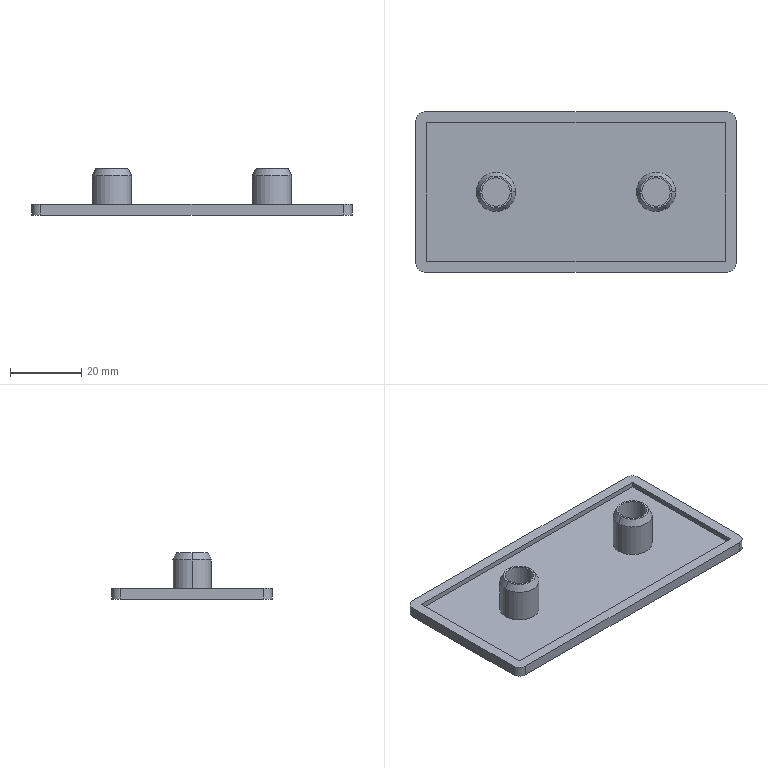Part | STEP file | HFC8_4590_Bc | 1 solid | 31 faces | box 90 x 45 x 13 mm | volume 8335 mm3 | plane 15 | cylinder 12 | cone 4 | commonest cylinder face diameters 5 x4 8 x4 11 x4
STEP:
#1=CARTESIAN_POINT('',(28.,0.,-1.5));
#2=VERTEX_POINT('',#1);
#3=CARTESIAN_POINT('',(17.,0.,-1.5));
#4=VERTEX_POINT('',#3);
#5=CARTESIAN_POINT('',(22.5,0.,-1.5));
#6=DIRECTION('',(0.,0.,1.));
#7=DIRECTION('',(1.,0.,0.));
#8=AXIS2_PLACEMENT_3D('',#5,#6,#7);
#9=CIRCLE('',#8,5.5);
#10=EDGE_CURVE('',#2,#4,#9,.T.);
#11=ORIENTED_EDGE('',*,*,#10,.T.);
#12=CARTESIAN_POINT('',(17.,0.,8.));
#13=VERTEX_POINT('',#12);
#14=CARTESIAN_POINT('',(17.,0.,-1.5));
#15=DIRECTION('',(0.,0.,1.));
#16=VECTOR('',#15,1000.);
#17=LINE('',#14,#16);
#18=EDGE_CURVE('',#4,#13,#17,.T.);
#19=ORIENTED_EDGE('',*,*,#18,.T.);
#20=CARTESIAN_POINT('',(28.,0.,8.));
#21=VERTEX_POINT('',#20);
#22=CARTESIAN_POINT('',(22.5,0.,8.));
#23=DIRECTION('',(0.,0.,1.));
#24=DIRECTION('',(1.,0.,0.));
#25=AXIS2_PLACEMENT_3D('',#22,#23,#24);
#26=CIRCLE('',#25,5.5);
#27=EDGE_CURVE('',#21,#13,#26,.T.);
#28=ORIENTED_EDGE('',*,*,#27,.F.);
#29=CARTESIAN_POINT('',(28.,0.,-1.5));
#30=DIRECTION('',(0.,0.,1.));
#31=VECTOR('',#30,1000.);
#32=LINE('',#29,#31);
#33=EDGE_CURVE('',#2,#21,#32,.T.);
#34=ORIENTED_EDGE('',*,*,#33,.F.);
#35=EDGE_LOOP('',(#11,#19,#28,#34));
#36=FACE_OUTER_BOUND('',#35,.T.);
#37=CARTESIAN_POINT('',(22.5,0.,-1.5));
#38=DIRECTION('',(0.,0.,1.));
#39=DIRECTION('',(1.,0.,0.));
#40=AXIS2_PLACEMENT_3D('',#37,#38,#39);
#41=CYLINDRICAL_SURFACE('',#40,5.5);
#42=ADVANCED_FACE('',(#36),#41,.T.);
#43=CARTESIAN_POINT('',(27.,0.,10.));
#44=VERTEX_POINT('',#43);
#45=CARTESIAN_POINT('',(18.,0.,10.));
#46=VERTEX_POINT('',#45);
#47=CARTESIAN_POINT('',(22.5,0.,10.));
#48=DIRECTION('',(0.,0.,1.));
#49=DIRECTION('',(1.,0.,0.));
#50=AXIS2_PLACEMENT_3D('',#47,#48,#49);
#51=CIRCLE('',#50,4.5);
#52=EDGE_CURVE('',#44,#46,#51,.T.);
#53=ORIENTED_EDGE('',*,*,#52,.F.);
#54=CARTESIAN_POINT('',(28.,0.,8.));
#55=DIRECTION('',(0.4472,0.,-0.8944));
#56=VECTOR('',#55,1000.);
#57=LINE('',#54,#56);
#58=EDGE_CURVE('',#44,#21,#57,.T.);
#59=ORIENTED_EDGE('',*,*,#58,.T.);
#60=ORIENTED_EDGE('',*,*,#27,.T.);
#61=CARTESIAN_POINT('',(17.,0.,8.));
#62=DIRECTION('',(-0.4472,0.,-0.8944));
#63=VECTOR('',#62,1000.);
#64=LINE('',#61,#63);
#65=EDGE_CURVE('',#46,#13,#64,.T.);
#66=ORIENTED_EDGE('',*,*,#65,.F.);
#67=EDGE_LOOP('',(#53,#59,#60,#66));
#68=FACE_OUTER_BOUND('',#67,.T.);
#69=CARTESIAN_POINT('',(22.5,0.,8.));
#70=DIRECTION('',(0.,0.,-1.));
#71=DIRECTION('',(-1.,0.,0.));
#72=AXIS2_PLACEMENT_3D('',#69,#70,#71);
#73=CONICAL_SURFACE('',#72,5.5,0.4636);
#74=ADVANCED_FACE('',(#68),#73,.T.);
#75=CARTESIAN_POINT('',(18.5,0.,0.));
#76=VERTEX_POINT('',#75);
#77=CARTESIAN_POINT('',(26.5,0.,0.));
#78=VERTEX_POINT('',#77);
#79=CARTESIAN_POINT('',(22.5,0.,0.));
#80=DIRECTION('',(0.,0.,1.));
#81=DIRECTION('',(1.,0.,0.));
#82=AXIS2_PLACEMENT_3D('',#79,#80,#81);
#83=CIRCLE('',#82,4.);
#84=EDGE_CURVE('',#76,#78,#83,.T.);
#85=ORIENTED_EDGE('',*,*,#84,.F.);
#86=CARTESIAN_POINT('',(18.5,0.,10.));
#87=VERTEX_POINT('',#86);
#88=CARTESIAN_POINT('',(18.5,0.,-1.5));
#89=DIRECTION('',(0.,0.,1.));
#90=VECTOR('',#89,1000.);
#91=LINE('',#88,#90);
#92=EDGE_CURVE('',#76,#87,#91,.T.);
#93=ORIENTED_EDGE('',*,*,#92,.T.);
#94=CARTESIAN_POINT('',(26.5,0.,10.));
#95=VERTEX_POINT('',#94);
#96=CARTESIAN_POINT('',(22.5,0.,10.));
#97=DIRECTION('',(0.,0.,1.));
#98=DIRECTION('',(1.,0.,0.));
#99=AXIS2_PLACEMENT_3D('',#96,#97,#98);
#100=CIRCLE('',#99,4.);
#101=EDGE_CURVE('',#87,#95,#100,.T.);
#102=ORIENTED_EDGE('',*,*,#101,.T.);
#103=CARTESIAN_POINT('',(26.5,0.,-1.5));
#104=DIRECTION('',(0.,0.,1.));
#105=VECTOR('',#104,1000.);
#106=LINE('',#103,#105);
#107=EDGE_CURVE('',#78,#95,#106,.T.);
#108=ORIENTED_EDGE('',*,*,#107,.F.);
#109=EDGE_LOOP('',(#85,#93,#102,#108));
#110=FACE_OUTER_BOUND('',#109,.T.);
#111=CARTESIAN_POINT('',(22.5,0.,-1.5));
#112=DIRECTION('',(0.,0.,1.));
#113=DIRECTION('',(1.,0.,0.));
#114=AXIS2_PLACEMENT_3D('',#111,#112,#113);
#115=CYLINDRICAL_SURFACE('',#114,4.);
#116=ADVANCED_FACE('',(#110),#115,.F.);
#117=CARTESIAN_POINT('',(-17.,0.,-1.5));
#118=VERTEX_POINT('',#117);
#119=CARTESIAN_POINT('',(-28.,0.,-1.5));
#120=VERTEX_POINT('',#119);
#121=CARTESIAN_POINT('',(-22.5,0.,-1.5));
#122=DIRECTION('',(0.,0.,1.));
#123=DIRECTION('',(1.,0.,0.));
#124=AXIS2_PLACEMENT_3D('',#121,#122,#123);
#125=CIRCLE('',#124,5.5);
#126=EDGE_CURVE('',#118,#120,#125,.T.);
#127=ORIENTED_EDGE('',*,*,#126,.T.);
#128=CARTESIAN_POINT('',(-28.,0.,8.));
#129=VERTEX_POINT('',#128);
#130=CARTESIAN_POINT('',(-28.,0.,-1.5));
#131=DIRECTION('',(0.,0.,1.));
#132=VECTOR('',#131,1000.);
#133=LINE('',#130,#132);
#134=EDGE_CURVE('',#120,#129,#133,.T.);
#135=ORIENTED_EDGE('',*,*,#134,.T.);
#136=CARTESIAN_POINT('',(-17.,0.,8.));
#137=VERTEX_POINT('',#136);
#138=CARTESIAN_POINT('',(-22.5,0.,8.));
#139=DIRECTION('',(0.,0.,1.));
#140=DIRECTION('',(1.,0.,0.));
#141=AXIS2_PLACEMENT_3D('',#138,#139,#140);
#142=CIRCLE('',#141,5.5);
#143=EDGE_CURVE('',#137,#129,#142,.T.);
#144=ORIENTED_EDGE('',*,*,#143,.F.);
#145=CARTESIAN_POINT('',(-17.,0.,-1.5));
#146=DIRECTION('',(0.,0.,1.));
#147=VECTOR('',#146,1000.);
#148=LINE('',#145,#147);
#149=EDGE_CURVE('',#118,#137,#148,.T.);
#150=ORIENTED_EDGE('',*,*,#149,.F.);
#151=EDGE_LOOP('',(#127,#135,#144,#150));
#152=FACE_OUTER_BOUND('',#151,.T.);
#153=CARTESIAN_POINT('',(-22.5,0.,-1.5));
#154=DIRECTION('',(0.,0.,1.));
#155=DIRECTION('',(1.,0.,0.));
#156=AXIS2_PLACEMENT_3D('',#153,#154,#155);
#157=CYLINDRICAL_SURFACE('',#156,5.5);
#158=ADVANCED_FACE('',(#152),#157,.T.);
#159=CARTESIAN_POINT('',(-18.,0.,10.));
#160=VERTEX_POINT('',#159);
#161=CARTESIAN_POINT('',(-27.,0.,10.));
#162=VERTEX_POINT('',#161);
#163=CARTESIAN_POINT('',(-22.5,0.,10.));
#164=DIRECTION('',(0.,0.,1.));
#165=DIRECTION('',(1.,0.,0.));
#166=AXIS2_PLACEMENT_3D('',#163,#164,#165);
#167=CIRCLE('',#166,4.5);
#168=EDGE_CURVE('',#160,#162,#167,.T.);
#169=ORIENTED_EDGE('',*,*,#168,.F.);
#170=CARTESIAN_POINT('',(-17.,0.,8.));
#171=DIRECTION('',(0.4472,0.,-0.8944));
#172=VECTOR('',#171,1000.);
#173=LINE('',#170,#172);
#174=EDGE_CURVE('',#160,#137,#173,.T.);
#175=ORIENTED_EDGE('',*,*,#174,.T.);
#176=ORIENTED_EDGE('',*,*,#143,.T.);
#177=CARTESIAN_POINT('',(-28.,0.,8.));
#178=DIRECTION('',(-0.4472,0.,-0.8944));
#179=VECTOR('',#178,1000.);
#180=LINE('',#177,#179);
#181=EDGE_CURVE('',#162,#129,#180,.T.);
#182=ORIENTED_EDGE('',*,*,#181,.F.);
#183=EDGE_LOOP('',(#169,#175,#176,#182));
#184=FACE_OUTER_BOUND('',#183,.T.);
#185=CARTESIAN_POINT('',(-22.5,0.,8.));
#186=DIRECTION('',(0.,0.,-1.));
#187=DIRECTION('',(-1.,0.,0.));
#188=AXIS2_PLACEMENT_3D('',#185,#186,#187);
#189=CONICAL_SURFACE('',#188,5.5,0.4636);
#190=ADVANCED_FACE('',(#184),#189,.T.);
#191=CARTESIAN_POINT('',(-26.5,0.,0.));
#192=VERTEX_POINT('',#191);
#193=CARTESIAN_POINT('',(-18.5,0.,0.));
#194=VERTEX_POINT('',#193);
#195=CARTESIAN_POINT('',(-22.5,0.,0.));
#196=DIRECTION('',(0.,0.,1.));
#197=DIRECTION('',(1.,0.,0.));
#198=AXIS2_PLACEMENT_3D('',#195,#196,#197);
#199=CIRCLE('',#198,4.);
#200=EDGE_CURVE('',#192,#194,#199,.T.);
#201=ORIENTED_EDGE('',*,*,#200,.F.);
#202=CARTESIAN_POINT('',(-26.5,0.,10.));
#203=VERTEX_POINT('',#202);
#204=CARTESIAN_POINT('',(-26.5,0.,-1.5));
#205=DIRECTION('',(0.,0.,1.));
#206=VECTOR('',#205,1000.);
#207=LINE('',#204,#206);
#208=EDGE_CURVE('',#192,#203,#207,.T.);
#209=ORIENTED_EDGE('',*,*,#208,.T.);
#210=CARTESIAN_POINT('',(-18.5,0.,10.));
#211=VERTEX_POINT('',#210);
#212=CARTESIAN_POINT('',(-22.5,0.,10.));
#213=DIRECTION('',(0.,0.,1.));
#214=DIRECTION('',(1.,0.,0.));
#215=AXIS2_PLACEMENT_3D('',#212,#213,#214);
#216=CIRCLE('',#215,4.);
#217=EDGE_CURVE('',#203,#211,#216,.T.);
#218=ORIENTED_EDGE('',*,*,#217,.T.);
#219=CARTESIAN_POINT('',(-18.5,0.,-1.5));
#220=DIRECTION('',(0.,0.,1.));
#221=VECTOR('',#220,1000.);
#222=LINE('',#219,#221);
#223=EDGE_CURVE('',#194,#211,#222,.T.);
#224=ORIENTED_EDGE('',*,*,#223,.F.);
#225=EDGE_LOOP('',(#201,#209,#218,#224));
#226=FACE_OUTER_BOUND('',#225,.T.);
#227=CARTESIAN_POINT('',(-22.5,0.,-1.5));
#228=DIRECTION('',(0.,0.,1.));
#229=DIRECTION('',(1.,0.,0.));
#230=AXIS2_PLACEMENT_3D('',#227,#228,#229);
#231=CYLINDRICAL_SURFACE('',#230,4.);
#232=ADVANCED_FACE('',(#226),#231,.F.);
#233=ORIENTED_EDGE('',*,*,#126,.F.);
#234=CARTESIAN_POINT('',(-22.5,0.,-1.5));
#235=DIRECTION('',(0.,0.,1.));
#236=DIRECTION('',(1.,0.,0.));
#237=AXIS2_PLACEMENT_3D('',#234,#235,#236);
#238=CIRCLE('',#237,5.5);
#239=EDGE_CURVE('',#120,#118,#238,.T.);
#240=ORIENTED_EDGE('',*,*,#239,.F.);
#241=EDGE_LOOP('',(#233,#240));
#242=FACE_BOUND('',#241,.T.);
#243=CARTESIAN_POINT('',(-42.,19.5,-1.5));
#244=VERTEX_POINT('',#243);
#245=CARTESIAN_POINT('',(-42.,-19.5,-1.5));
#246=VERTEX_POINT('',#245);
#247=CARTESIAN_POINT('',(-42.,19.5,-1.5));
#248=DIRECTION('',(0.,-1.,0.));
#249=VECTOR('',#248,1000.);
#250=LINE('',#247,#249);
#251=EDGE_CURVE('',#244,#246,#250,.T.);
#252=ORIENTED_EDGE('',*,*,#251,.T.);
#253=CARTESIAN_POINT('',(42.,-19.5,-1.5));
#254=VERTEX_POINT('',#253);
#255=CARTESIAN_POINT('',(-42.,-19.5,-1.5));
#256=DIRECTION('',(1.,0.,0.));
#257=VECTOR('',#256,1000.);
#258=LINE('',#255,#257);
#259=EDGE_CURVE('',#246,#254,#258,.T.);
#260=ORIENTED_EDGE('',*,*,#259,.T.);
#261=CARTESIAN_POINT('',(42.,19.5,-1.5));
#262=VERTEX_POINT('',#261);
#263=CARTESIAN_POINT('',(42.,-19.5,-1.5));
#264=DIRECTION('',(0.,1.,0.));
#265=VECTOR('',#264,1000.);
#266=LINE('',#263,#265);
#267=EDGE_CURVE('',#254,#262,#266,.T.);
#268=ORIENTED_EDGE('',*,*,#267,.T.);
#269=CARTESIAN_POINT('',(42.,19.5,-1.5));
#270=DIRECTION('',(-1.,0.,0.));
#271=VECTOR('',#270,1000.);
#272=LINE('',#269,#271);
#273=EDGE_CURVE('',#262,#244,#272,.T.);
#274=ORIENTED_EDGE('',*,*,#273,.T.);
#275=EDGE_LOOP('',(#252,#260,#268,#274));
#276=FACE_OUTER_BOUND('',#275,.T.);
#277=ORIENTED_EDGE('',*,*,#10,.F.);
#278=CARTESIAN_POINT('',(22.5,0.,-1.5));
#279=DIRECTION('',(0.,0.,1.));
#280=DIRECTION('',(1.,0.,0.));
#281=AXIS2_PLACEMENT_3D('',#278,#279,#280);
#282=CIRCLE('',#281,5.5);
#283=EDGE_CURVE('',#4,#2,#282,.T.);
#284=ORIENTED_EDGE('',*,*,#283,.F.);
#285=EDGE_LOOP('',(#277,#284));
#286=FACE_BOUND('',#285,.T.);
#287=CARTESIAN_POINT('',(-42.,-19.5,-1.5));
#288=DIRECTION('',(0.,0.,1.));
#289=DIRECTION('',(1.,0.,0.));
#290=AXIS2_PLACEMENT_3D('',#287,#288,#289);
#291=PLANE('',#290);
#292=ADVANCED_FACE('',(#242,#276,#286),#291,.T.);
#293=CARTESIAN_POINT('',(-42.5,22.5,0.));
#294=VERTEX_POINT('',#293);
#295=CARTESIAN_POINT('',(-45.,20.,0.));
#296=VERTEX_POINT('',#295);
#297=CARTESIAN_POINT('',(-42.5,20.,0.));
#298=DIRECTION('',(0.,0.,1.));
#299=DIRECTION('',(1.,0.,0.));
#300=AXIS2_PLACEMENT_3D('',#297,#298,#299);
#301=CIRCLE('',#300,2.5);
#302=EDGE_CURVE('',#294,#296,#301,.T.);
#303=ORIENTED_EDGE('',*,*,#302,.F.);
#304=CARTESIAN_POINT('',(-42.5,22.5,-3.));
#305=VERTEX_POINT('',#304);
#306=CARTESIAN_POINT('',(-42.5,22.5,-3.));
#307=DIRECTION('',(0.,0.,1.));
#308=VECTOR('',#307,1000.);
#309=LINE('',#306,#308);
#310=EDGE_CURVE('',#305,#294,#309,.T.);
#311=ORIENTED_EDGE('',*,*,#310,.F.);
#312=CARTESIAN_POINT('',(-45.,20.,-3.));
#313=VERTEX_POINT('',#312);
#314=CARTESIAN_POINT('',(-42.5,20.,-3.));
#315=DIRECTION('',(0.,0.,1.));
#316=DIRECTION('',(1.,0.,0.));
#317=AXIS2_PLACEMENT_3D('',#314,#315,#316);
#318=CIRCLE('',#317,2.5);
#319=EDGE_CURVE('',#305,#313,#318,.T.);
#320=ORIENTED_EDGE('',*,*,#319,.T.);
#321=CARTESIAN_POINT('',(-45.,20.,-3.));
#322=DIRECTION('',(0.,0.,1.));
#323=VECTOR('',#322,1000.);
#324=LINE('',#321,#323);
#325=EDGE_CURVE('',#313,#296,#324,.T.);
#326=ORIENTED_EDGE('',*,*,#325,.T.);
#327=EDGE_LOOP('',(#303,#311,#320,#326));
#328=FACE_OUTER_BOUND('',#327,.T.);
#329=CARTESIAN_POINT('',(-42.5,20.,-3.));
#330=DIRECTION('',(0.,0.,1.));
#331=DIRECTION('',(1.,0.,0.));
#332=AXIS2_PLACEMENT_3D('',#329,#330,#331);
#333=CYLINDRICAL_SURFACE('',#332,2.5);
#334=ADVANCED_FACE('',(#328),#333,.T.);
#335=CARTESIAN_POINT('',(42.5,22.5,0.));
#336=VERTEX_POINT('',#335);
#337=CARTESIAN_POINT('',(42.5,22.5,0.));
#338=DIRECTION('',(-1.,0.,0.));
#339=VECTOR('',#338,1000.);
#340=LINE('',#337,#339);
#341=EDGE_CURVE('',#336,#294,#340,.T.);
#342=ORIENTED_EDGE('',*,*,#341,.F.);
#343=CARTESIAN_POINT('',(42.5,22.5,-3.));
#344=VERTEX_POINT('',#343);
#345=CARTESIAN_POINT('',(42.5,22.5,-3.));
#346=DIRECTION('',(0.,0.,1.));
#347=VECTOR('',#346,1000.);
#348=LINE('',#345,#347);
#349=EDGE_CURVE('',#344,#336,#348,.T.);
#350=ORIENTED_EDGE('',*,*,#349,.F.);
#351=CARTESIAN_POINT('',(42.5,22.5,-3.));
#352=DIRECTION('',(-1.,0.,0.));
#353=VECTOR('',#352,1000.);
#354=LINE('',#351,#353);
#355=EDGE_CURVE('',#344,#305,#354,.T.);
#356=ORIENTED_EDGE('',*,*,#355,.T.);
#357=ORIENTED_EDGE('',*,*,#310,.T.);
#358=EDGE_LOOP('',(#342,#350,#356,#357));
#359=FACE_OUTER_BOUND('',#358,.T.);
#360=CARTESIAN_POINT('',(42.5,22.5,-3.));
#361=DIRECTION('',(0.,1.,0.));
#362=DIRECTION('',(0.,0.,1.));
#363=AXIS2_PLACEMENT_3D('',#360,#361,#362);
#364=PLANE('',#363);
#365=ADVANCED_FACE('',(#359),#364,.T.);
#366=CARTESIAN_POINT('',(45.,20.,0.));
#367=VERTEX_POINT('',#366);
#368=CARTESIAN_POINT('',(42.5,20.,0.));
#369=DIRECTION('',(0.,0.,1.));
#370=DIRECTION('',(1.,0.,0.));
#371=AXIS2_PLACEMENT_3D('',#368,#369,#370);
#372=CIRCLE('',#371,2.5);
#373=EDGE_CURVE('',#367,#336,#372,.T.);
#374=ORIENTED_EDGE('',*,*,#373,.F.);
#375=CARTESIAN_POINT('',(45.,20.,-3.));
#376=VERTEX_POINT('',#375);
#377=CARTESIAN_POINT('',(45.,20.,-3.));
#378=DIRECTION('',(0.,0.,1.));
#379=VECTOR('',#378,1000.);
#380=LINE('',#377,#379);
#381=EDGE_CURVE('',#376,#367,#380,.T.);
#382=ORIENTED_EDGE('',*,*,#381,.F.);
#383=CARTESIAN_POINT('',(42.5,20.,-3.));
#384=DIRECTION('',(0.,0.,1.));
#385=DIRECTION('',(1.,0.,0.));
#386=AXIS2_PLACEMENT_3D('',#383,#384,#385);
#387=CIRCLE('',#386,2.5);
#388=EDGE_CURVE('',#376,#344,#387,.T.);
#389=ORIENTED_EDGE('',*,*,#388,.T.);
#390=ORIENTED_EDGE('',*,*,#349,.T.);
#391=EDGE_LOOP('',(#374,#382,#389,#390));
#392=FACE_OUTER_BOUND('',#391,.T.);
#393=CARTESIAN_POINT('',(42.5,20.,-3.));
#394=DIRECTION('',(0.,0.,1.));
#395=DIRECTION('',(1.,0.,0.));
#396=AXIS2_PLACEMENT_3D('',#393,#394,#395);
#397=CYLINDRICAL_SURFACE('',#396,2.5);
#398=ADVANCED_FACE('',(#392),#397,.T.);
#399=CARTESIAN_POINT('',(45.,-20.,0.));
#400=VERTEX_POINT('',#399);
#401=CARTESIAN_POINT('',(45.,-20.,0.));
#402=DIRECTION('',(0.,1.,0.));
#403=VECTOR('',#402,1000.);
#404=LINE('',#401,#403);
#405=EDGE_CURVE('',#400,#367,#404,.T.);
#406=ORIENTED_EDGE('',*,*,#405,.F.);
#407=CARTESIAN_POINT('',(45.,-20.,-3.));
#408=VERTEX_POINT('',#407);
#409=CARTESIAN_POINT('',(45.,-20.,-3.));
#410=DIRECTION('',(0.,0.,1.));
#411=VECTOR('',#410,1000.);
#412=LINE('',#409,#411);
#413=EDGE_CURVE('',#408,#400,#412,.T.);
#414=ORIENTED_EDGE('',*,*,#413,.F.);
#415=CARTESIAN_POINT('',(45.,-20.,-3.));
#416=DIRECTION('',(0.,1.,0.));
#417=VECTOR('',#416,1000.);
#418=LINE('',#415,#417);
#419=EDGE_CURVE('',#408,#376,#418,.T.);
#420=ORIENTED_EDGE('',*,*,#419,.T.);
#421=ORIENTED_EDGE('',*,*,#381,.T.);
#422=EDGE_LOOP('',(#406,#414,#420,#421));
#423=FACE_OUTER_BOUND('',#422,.T.);
#424=CARTESIAN_POINT('',(45.,-20.,-3.));
#425=DIRECTION('',(1.,0.,0.));
#426=DIRECTION('',(0.,0.,-1.));
#427=AXIS2_PLACEMENT_3D('',#424,#425,#426);
#428=PLANE('',#427);
#429=ADVANCED_FACE('',(#423),#428,.T.);
#430=CARTESIAN_POINT('',(42.5,-22.5,0.));
#431=VERTEX_POINT('',#430);
#432=CARTESIAN_POINT('',(42.5,-20.,0.));
#433=DIRECTION('',(0.,0.,1.));
#434=DIRECTION('',(1.,0.,0.));
#435=AXIS2_PLACEMENT_3D('',#432,#433,#434);
#436=CIRCLE('',#435,2.5);
#437=EDGE_CURVE('',#431,#400,#436,.T.);
#438=ORIENTED_EDGE('',*,*,#437,.F.);
#439=CARTESIAN_POINT('',(42.5,-22.5,-3.));
#440=VERTEX_POINT('',#439);
#441=CARTESIAN_POINT('',(42.5,-22.5,-3.));
#442=DIRECTION('',(0.,0.,1.));
#443=VECTOR('',#442,1000.);
#444=LINE('',#441,#443);
#445=EDGE_CURVE('',#440,#431,#444,.T.);
#446=ORIENTED_EDGE('',*,*,#445,.F.);
#447=CARTESIAN_POINT('',(42.5,-20.,-3.));
#448=DIRECTION('',(0.,0.,1.));
#449=DIRECTION('',(1.,0.,0.));
#450=AXIS2_PLACEMENT_3D('',#447,#448,#449);
#451=CIRCLE('',#450,2.5);
#452=EDGE_CURVE('',#440,#408,#451,.T.);
#453=ORIENTED_EDGE('',*,*,#452,.T.);
#454=ORIENTED_EDGE('',*,*,#413,.T.);
#455=EDGE_LOOP('',(#438,#446,#453,#454));
#456=FACE_OUTER_BOUND('',#455,.T.);
#457=CARTESIAN_POINT('',(42.5,-20.,-3.));
#458=DIRECTION('',(0.,0.,1.));
#459=DIRECTION('',(1.,0.,0.));
#460=AXIS2_PLACEMENT_3D('',#457,#458,#459);
#461=CYLINDRICAL_SURFACE('',#460,2.5);
#462=ADVANCED_FACE('',(#456),#461,.T.);
#463=CARTESIAN_POINT('',(-42.5,-22.5,0.));
#464=VERTEX_POINT('',#463);
#465=CARTESIAN_POINT('',(-42.5,-22.5,0.));
#466=DIRECTION('',(1.,0.,0.));
#467=VECTOR('',#466,1000.);
#468=LINE('',#465,#467);
#469=EDGE_CURVE('',#464,#431,#468,.T.);
#470=ORIENTED_EDGE('',*,*,#469,.F.);
#471=CARTESIAN_POINT('',(-42.5,-22.5,-3.));
#472=VERTEX_POINT('',#471);
#473=CARTESIAN_POINT('',(-42.5,-22.5,-3.));
#474=DIRECTION('',(0.,0.,1.));
#475=VECTOR('',#474,1000.);
#476=LINE('',#473,#475);
#477=EDGE_CURVE('',#472,#464,#476,.T.);
#478=ORIENTED_EDGE('',*,*,#477,.F.);
#479=CARTESIAN_POINT('',(-42.5,-22.5,-3.));
#480=DIRECTION('',(1.,0.,0.));
#481=VECTOR('',#480,1000.);
#482=LINE('',#479,#481);
#483=EDGE_CURVE('',#472,#440,#482,.T.);
#484=ORIENTED_EDGE('',*,*,#483,.T.);
#485=ORIENTED_EDGE('',*,*,#445,.T.);
#486=EDGE_LOOP('',(#470,#478,#484,#485));
#487=FACE_OUTER_BOUND('',#486,.T.);
#488=CARTESIAN_POINT('',(-42.5,-22.5,-3.));
#489=DIRECTION('',(0.,-1.,0.));
#490=DIRECTION('',(0.,0.,-1.));
#491=AXIS2_PLACEMENT_3D('',#488,#489,#490);
#492=PLANE('',#491);
#493=ADVANCED_FACE('',(#487),#492,.T.);
#494=CARTESIAN_POINT('',(-45.,-20.,0.));
#495=VERTEX_POINT('',#494);
#496=CARTESIAN_POINT('',(-42.5,-20.,0.));
#497=DIRECTION('',(0.,0.,1.));
#498=DIRECTION('',(1.,0.,0.));
#499=AXIS2_PLACEMENT_3D('',#496,#497,#498);
#500=CIRCLE('',#499,2.5);
#501=EDGE_CURVE('',#495,#464,#500,.T.);
#502=ORIENTED_EDGE('',*,*,#501,.F.);
#503=CARTESIAN_POINT('',(-45.,-20.,-3.));
#504=VERTEX_POINT('',#503);
#505=CARTESIAN_POINT('',(-45.,-20.,-3.));
#506=DIRECTION('',(0.,0.,1.));
#507=VECTOR('',#506,1000.);
#508=LINE('',#505,#507);
#509=EDGE_CURVE('',#504,#495,#508,.T.);
#510=ORIENTED_EDGE('',*,*,#509,.F.);
#511=CARTESIAN_POINT('',(-42.5,-20.,-3.));
#512=DIRECTION('',(0.,0.,1.));
#513=DIRECTION('',(1.,0.,0.));
#514=AXIS2_PLACEMENT_3D('',#511,#512,#513);
#515=CIRCLE('',#514,2.5);
#516=EDGE_CURVE('',#504,#472,#515,.T.);
#517=ORIENTED_EDGE('',*,*,#516,.T.);
#518=ORIENTED_EDGE('',*,*,#477,.T.);
#519=EDGE_LOOP('',(#502,#510,#517,#518));
#520=FACE_OUTER_BOUND('',#519,.T.);
#521=CARTESIAN_POINT('',(-42.5,-20.,-3.));
#522=DIRECTION('',(0.,0.,1.));
#523=DIRECTION('',(1.,0.,0.));
#524=AXIS2_PLACEMENT_3D('',#521,#522,#523);
#525=CYLINDRICAL_SURFACE('',#524,2.5);
#526=ADVANCED_FACE('',(#520),#525,.T.);
#527=CARTESIAN_POINT('',(-45.,20.,0.));
#528=DIRECTION('',(0.,-1.,0.));
#529=VECTOR('',#528,1000.);
#530=LINE('',#527,#529);
#531=EDGE_CURVE('',#296,#495,#530,.T.);
#532=ORIENTED_EDGE('',*,*,#531,.F.);
#533=ORIENTED_EDGE('',*,*,#325,.F.);
#534=CARTESIAN_POINT('',(-45.,20.,-3.));
#535=DIRECTION('',(0.,-1.,0.));
#536=VECTOR('',#535,1000.);
#537=LINE('',#534,#536);
#538=EDGE_CURVE('',#313,#504,#537,.T.);
#539=ORIENTED_EDGE('',*,*,#538,.T.);
#540=ORIENTED_EDGE('',*,*,#509,.T.);
#541=EDGE_LOOP('',(#532,#533,#539,#540));
#542=FACE_OUTER_BOUND('',#541,.T.);
#543=CARTESIAN_POINT('',(-45.,20.,-3.));
#544=DIRECTION('',(-1.,0.,0.));
#545=DIRECTION('',(0.,0.,1.));
#546=AXIS2_PLACEMENT_3D('',#543,#544,#545);
#547=PLANE('',#546);
#548=ADVANCED_FACE('',(#542),#547,.T.);
#549=ORIENTED_EDGE('',*,*,#319,.F.);
#550=ORIENTED_EDGE('',*,*,#355,.F.);
#551=ORIENTED_EDGE('',*,*,#388,.F.);
#552=ORIENTED_EDGE('',*,*,#419,.F.);
#553=ORIENTED_EDGE('',*,*,#452,.F.);
#554=ORIENTED_EDGE('',*,*,#483,.F.);
#555=ORIENTED_EDGE('',*,*,#516,.F.);
#556=ORIENTED_EDGE('',*,*,#538,.F.);
#557=EDGE_LOOP('',(#549,#550,#551,#552,#553,#554,#555,#556));
#558=FACE_OUTER_BOUND('',#557,.T.);
#559=CARTESIAN_POINT('',(-42.5,20.,-3.));
#560=DIRECTION('',(0.,0.,1.));
#561=DIRECTION('',(1.,0.,0.));
#562=AXIS2_PLACEMENT_3D('',#559,#560,#561);
#563=PLANE('',#562);
#564=ADVANCED_FACE('',(#558),#563,.F.);
#565=CARTESIAN_POINT('',(-42.,19.5,0.));
#566=VERTEX_POINT('',#565);
#567=CARTESIAN_POINT('',(-42.,-19.5,0.));
#568=VERTEX_POINT('',#567);
#569=CARTESIAN_POINT('',(-42.,19.5,0.));
#570=DIRECTION('',(0.,-1.,0.));
#571=VECTOR('',#570,1000.);
#572=LINE('',#569,#571);
#573=EDGE_CURVE('',#566,#568,#572,.T.);
#574=ORIENTED_EDGE('',*,*,#573,.F.);
#575=CARTESIAN_POINT('',(42.,19.5,0.));
#576=VERTEX_POINT('',#575);
#577=CARTESIAN_POINT('',(42.,19.5,0.));
#578=DIRECTION('',(-1.,0.,0.));
#579=VECTOR('',#578,1000.);
#580=LINE('',#577,#579);
#581=EDGE_CURVE('',#576,#566,#580,.T.);
#582=ORIENTED_EDGE('',*,*,#581,.F.);
#583=CARTESIAN_POINT('',(42.,-19.5,0.));
#584=VERTEX_POINT('',#583);
#585=CARTESIAN_POINT('',(42.,-19.5,0.));
#586=DIRECTION('',(0.,1.,0.));
#587=VECTOR('',#586,1000.);
#588=LINE('',#585,#587);
#589=EDGE_CURVE('',#584,#576,#588,.T.);
#590=ORIENTED_EDGE('',*,*,#589,.F.);
#591=CARTESIAN_POINT('',(-42.,-19.5,0.));
#592=DIRECTION('',(1.,0.,0.));
#593=VECTOR('',#592,1000.);
#594=LINE('',#591,#593);
#595=EDGE_CURVE('',#568,#584,#594,.T.);
#596=ORIENTED_EDGE('',*,*,#595,.F.);
#597=EDGE_LOOP('',(#574,#582,#590,#596));
#598=FACE_BOUND('',#597,.T.);
#599=ORIENTED_EDGE('',*,*,#302,.T.);
#600=ORIENTED_EDGE('',*,*,#531,.T.);
#601=ORIENTED_EDGE('',*,*,#501,.T.);
#602=ORIENTED_EDGE('',*,*,#469,.T.);
#603=ORIENTED_EDGE('',*,*,#437,.T.);
#604=ORIENTED_EDGE('',*,*,#405,.T.);
#605=ORIENTED_EDGE('',*,*,#373,.T.);
#606=ORIENTED_EDGE('',*,*,#341,.T.);
#607=EDGE_LOOP('',(#599,#600,#601,#602,#603,#604,#605,#606));
#608=FACE_OUTER_BOUND('',#607,.T.);
#609=CARTESIAN_POINT('',(-42.5,20.,0.));
#610=DIRECTION('',(0.,0.,1.));
#611=DIRECTION('',(1.,0.,0.));
#612=AXIS2_PLACEMENT_3D('',#609,#610,#611);
#613=PLANE('',#612);
#614=ADVANCED_FACE('',(#598,#608),#613,.T.);
#615=ORIENTED_EDGE('',*,*,#573,.T.);
#616=CARTESIAN_POINT('',(-42.,-19.5,-1.5));
#617=DIRECTION('',(0.,0.,1.));
#618=VECTOR('',#617,1000.);
#619=LINE('',#616,#618);
#620=EDGE_CURVE('',#246,#568,#619,.T.);
#621=ORIENTED_EDGE('',*,*,#620,.F.);
#622=ORIENTED_EDGE('',*,*,#251,.F.);
#623=CARTESIAN_POINT('',(-42.,19.5,-1.5));
#624=DIRECTION('',(0.,0.,1.));
#625=VECTOR('',#624,1000.);
#626=LINE('',#623,#625);
#627=EDGE_CURVE('',#244,#566,#626,.T.);
#628=ORIENTED_EDGE('',*,*,#627,.T.);
#629=EDGE_LOOP('',(#615,#621,#622,#628));
#630=FACE_OUTER_BOUND('',#629,.T.);
#631=CARTESIAN_POINT('',(-42.,19.5,-1.5));
#632=DIRECTION('',(-1.,0.,0.));
#633=DIRECTION('',(0.,0.,1.));
#634=AXIS2_PLACEMENT_3D('',#631,#632,#633);
#635=PLANE('',#634);
#636=ADVANCED_FACE('',(#630),#635,.F.);
#637=ORIENTED_EDGE('',*,*,#581,.T.);
#638=ORIENTED_EDGE('',*,*,#627,.F.);
#639=ORIENTED_EDGE('',*,*,#273,.F.);
#640=CARTESIAN_POINT('',(42.,19.5,-1.5));
#641=DIRECTION('',(0.,0.,1.));
#642=VECTOR('',#641,1000.);
#643=LINE('',#640,#642);
#644=EDGE_CURVE('',#262,#576,#643,.T.);
#645=ORIENTED_EDGE('',*,*,#644,.T.);
#646=EDGE_LOOP('',(#637,#638,#639,#645));
#647=FACE_OUTER_BOUND('',#646,.T.);
#648=CARTESIAN_POINT('',(42.,19.5,-1.5));
#649=DIRECTION('',(0.,1.,0.));
#650=DIRECTION('',(0.,0.,1.));
#651=AXIS2_PLACEMENT_3D('',#648,#649,#650);
#652=PLANE('',#651);
#653=ADVANCED_FACE('',(#647),#652,.F.);
#654=ORIENTED_EDGE('',*,*,#589,.T.);
#655=ORIENTED_EDGE('',*,*,#644,.F.);
#656=ORIENTED_EDGE('',*,*,#267,.F.);
#657=CARTESIAN_POINT('',(42.,-19.5,-1.5));
#658=DIRECTION('',(0.,0.,1.));
#659=VECTOR('',#658,1000.);
#660=LINE('',#657,#659);
#661=EDGE_CURVE('',#254,#584,#660,.T.);
#662=ORIENTED_EDGE('',*,*,#661,.T.);
#663=EDGE_LOOP('',(#654,#655,#656,#662));
#664=FACE_OUTER_BOUND('',#663,.T.);
#665=CARTESIAN_POINT('',(42.,-19.5,-1.5));
#666=DIRECTION('',(1.,0.,0.));
#667=DIRECTION('',(0.,0.,-1.));
#668=AXIS2_PLACEMENT_3D('',#665,#666,#667);
#669=PLANE('',#668);
#670=ADVANCED_FACE('',(#664),#669,.F.);
#671=ORIENTED_EDGE('',*,*,#595,.T.);
#672=ORIENTED_EDGE('',*,*,#661,.F.);
#673=ORIENTED_EDGE('',*,*,#259,.F.);
#674=ORIENTED_EDGE('',*,*,#620,.T.);
#675=EDGE_LOOP('',(#671,#672,#673,#674));
#676=FACE_OUTER_BOUND('',#675,.T.);
#677=CARTESIAN_POINT('',(-42.,-19.5,-1.5));
#678=DIRECTION('',(0.,-1.,0.));
#679=DIRECTION('',(0.,0.,-1.));
#680=AXIS2_PLACEMENT_3D('',#677,#678,#679);
#681=PLANE('',#680);
#682=ADVANCED_FACE('',(#676),#681,.F.);
#683=CARTESIAN_POINT('',(-22.5,0.,0.));
#684=DIRECTION('',(0.,0.,1.));
#685=DIRECTION('',(1.,0.,0.));
#686=AXIS2_PLACEMENT_3D('',#683,#684,#685);
#687=CIRCLE('',#686,4.);
#688=EDGE_CURVE('',#194,#192,#687,.T.);
#689=ORIENTED_EDGE('',*,*,#688,.T.);
#690=ORIENTED_EDGE('',*,*,#200,.T.);
#691=EDGE_LOOP('',(#689,#690));
#692=FACE_OUTER_BOUND('',#691,.T.);
#693=CARTESIAN_POINT('',(-22.5,0.,0.));
#694=DIRECTION('',(0.,0.,-1.));
#695=DIRECTION('',(-1.,0.,0.));
#696=AXIS2_PLACEMENT_3D('',#693,#694,#695);
#697=PLANE('',#696);
#698=ADVANCED_FACE('',(#692),#697,.F.);
#699=ORIENTED_EDGE('',*,*,#208,.F.);
#700=ORIENTED_EDGE('',*,*,#688,.F.);
#701=ORIENTED_EDGE('',*,*,#223,.T.);
#702=CARTESIAN_POINT('',(-22.5,0.,10.));
#703=DIRECTION('',(0.,0.,1.));
#704=DIRECTION('',(1.,0.,0.));
#705=AXIS2_PLACEMENT_3D('',#702,#703,#704);
#706=CIRCLE('',#705,4.);
#707=EDGE_CURVE('',#211,#203,#706,.T.);
#708=ORIENTED_EDGE('',*,*,#707,.T.);
#709=EDGE_LOOP('',(#699,#700,#701,#708));
#710=FACE_OUTER_BOUND('',#709,.T.);
#711=CARTESIAN_POINT('',(-22.5,0.,-1.5));
#712=DIRECTION('',(0.,0.,1.));
#713=DIRECTION('',(1.,0.,0.));
#714=AXIS2_PLACEMENT_3D('',#711,#712,#713);
#715=CYLINDRICAL_SURFACE('',#714,4.);
#716=ADVANCED_FACE('',(#710),#715,.F.);
#717=ORIENTED_EDGE('',*,*,#707,.F.);
#718=ORIENTED_EDGE('',*,*,#217,.F.);
#719=EDGE_LOOP('',(#717,#718));
#720=FACE_BOUND('',#719,.T.);
#721=CARTESIAN_POINT('',(-22.5,0.,10.));
#722=DIRECTION('',(0.,0.,1.));
#723=DIRECTION('',(1.,0.,0.));
#724=AXIS2_PLACEMENT_3D('',#721,#722,#723);
#725=CIRCLE('',#724,4.5);
#726=EDGE_CURVE('',#162,#160,#725,.T.);
#727=ORIENTED_EDGE('',*,*,#726,.T.);
#728=ORIENTED_EDGE('',*,*,#168,.T.);
#729=EDGE_LOOP('',(#727,#728));
#730=FACE_OUTER_BOUND('',#729,.T.);
#731=CARTESIAN_POINT('',(-22.5,4.,10.));
#732=DIRECTION('',(0.,0.,-1.));
#733=DIRECTION('',(-1.,0.,0.));
#734=AXIS2_PLACEMENT_3D('',#731,#732,#733);
#735=PLANE('',#734);
#736=ADVANCED_FACE('',(#720,#730),#735,.F.);
#737=ORIENTED_EDGE('',*,*,#174,.F.);
#738=ORIENTED_EDGE('',*,*,#726,.F.);
#739=ORIENTED_EDGE('',*,*,#181,.T.);
#740=CARTESIAN_POINT('',(-22.5,0.,8.));
#741=DIRECTION('',(0.,0.,1.));
#742=DIRECTION('',(1.,0.,0.));
#743=AXIS2_PLACEMENT_3D('',#740,#741,#742);
#744=CIRCLE('',#743,5.5);
#745=EDGE_CURVE('',#129,#137,#744,.T.);
#746=ORIENTED_EDGE('',*,*,#745,.T.);
#747=EDGE_LOOP('',(#737,#738,#739,#746));
#748=FACE_OUTER_BOUND('',#747,.T.);
#749=CARTESIAN_POINT('',(-22.5,0.,8.));
#750=DIRECTION('',(0.,0.,-1.));
#751=DIRECTION('',(-1.,0.,0.));
#752=AXIS2_PLACEMENT_3D('',#749,#750,#751);
#753=CONICAL_SURFACE('',#752,5.5,0.4636);
#754=ADVANCED_FACE('',(#748),#753,.T.);
#755=ORIENTED_EDGE('',*,*,#134,.F.);
#756=ORIENTED_EDGE('',*,*,#239,.T.);
#757=ORIENTED_EDGE('',*,*,#149,.T.);
#758=ORIENTED_EDGE('',*,*,#745,.F.);
#759=EDGE_LOOP('',(#755,#756,#757,#758));
#760=FACE_OUTER_BOUND('',#759,.T.);
#761=CARTESIAN_POINT('',(-22.5,0.,-1.5));
#762=DIRECTION('',(0.,0.,1.));
#763=DIRECTION('',(1.,0.,0.));
#764=AXIS2_PLACEMENT_3D('',#761,#762,#763);
#765=CYLINDRICAL_SURFACE('',#764,5.5);
#766=ADVANCED_FACE('',(#760),#765,.T.);
#767=CARTESIAN_POINT('',(22.5,0.,0.));
#768=DIRECTION('',(0.,0.,1.));
#769=DIRECTION('',(1.,0.,0.));
#770=AXIS2_PLACEMENT_3D('',#767,#768,#769);
#771=CIRCLE('',#770,4.);
#772=EDGE_CURVE('',#78,#76,#771,.T.);
#773=ORIENTED_EDGE('',*,*,#772,.T.);
#774=ORIENTED_EDGE('',*,*,#84,.T.);
#775=EDGE_LOOP('',(#773,#774));
#776=FACE_OUTER_BOUND('',#775,.T.);
#777=CARTESIAN_POINT('',(22.5,0.,0.));
#778=DIRECTION('',(0.,0.,-1.));
#779=DIRECTION('',(-1.,0.,0.));
#780=AXIS2_PLACEMENT_3D('',#777,#778,#779);
#781=PLANE('',#780);
#782=ADVANCED_FACE('',(#776),#781,.F.);
#783=ORIENTED_EDGE('',*,*,#92,.F.);
#784=ORIENTED_EDGE('',*,*,#772,.F.);
#785=ORIENTED_EDGE('',*,*,#107,.T.);
#786=CARTESIAN_POINT('',(22.5,0.,10.));
#787=DIRECTION('',(0.,0.,1.));
#788=DIRECTION('',(1.,0.,0.));
#789=AXIS2_PLACEMENT_3D('',#786,#787,#788);
#790=CIRCLE('',#789,4.);
#791=EDGE_CURVE('',#95,#87,#790,.T.);
#792=ORIENTED_EDGE('',*,*,#791,.T.);
#793=EDGE_LOOP('',(#783,#784,#785,#792));
#794=FACE_OUTER_BOUND('',#793,.T.);
#795=CARTESIAN_POINT('',(22.5,0.,-1.5));
#796=DIRECTION('',(0.,0.,1.));
#797=DIRECTION('',(1.,0.,0.));
#798=AXIS2_PLACEMENT_3D('',#795,#796,#797);
#799=CYLINDRICAL_SURFACE('',#798,4.);
#800=ADVANCED_FACE('',(#794),#799,.F.);
#801=ORIENTED_EDGE('',*,*,#791,.F.);
#802=ORIENTED_EDGE('',*,*,#101,.F.);
#803=EDGE_LOOP('',(#801,#802));
#804=FACE_BOUND('',#803,.T.);
#805=CARTESIAN_POINT('',(22.5,0.,10.));
#806=DIRECTION('',(0.,0.,1.));
#807=DIRECTION('',(1.,0.,0.));
#808=AXIS2_PLACEMENT_3D('',#805,#806,#807);
#809=CIRCLE('',#808,4.5);
#810=EDGE_CURVE('',#46,#44,#809,.T.);
#811=ORIENTED_EDGE('',*,*,#810,.T.);
#812=ORIENTED_EDGE('',*,*,#52,.T.);
#813=EDGE_LOOP('',(#811,#812));
#814=FACE_OUTER_BOUND('',#813,.T.);
#815=CARTESIAN_POINT('',(22.5,4.,10.));
#816=DIRECTION('',(0.,0.,-1.));
#817=DIRECTION('',(-1.,0.,0.));
#818=AXIS2_PLACEMENT_3D('',#815,#816,#817);
#819=PLANE('',#818);
#820=ADVANCED_FACE('',(#804,#814),#819,.F.);
#821=ORIENTED_EDGE('',*,*,#58,.F.);
#822=ORIENTED_EDGE('',*,*,#810,.F.);
#823=ORIENTED_EDGE('',*,*,#65,.T.);
#824=CARTESIAN_POINT('',(22.5,0.,8.));
#825=DIRECTION('',(0.,0.,1.));
#826=DIRECTION('',(1.,0.,0.));
#827=AXIS2_PLACEMENT_3D('',#824,#825,#826);
#828=CIRCLE('',#827,5.5);
#829=EDGE_CURVE('',#13,#21,#828,.T.);
#830=ORIENTED_EDGE('',*,*,#829,.T.);
#831=EDGE_LOOP('',(#821,#822,#823,#830));
#832=FACE_OUTER_BOUND('',#831,.T.);
#833=CARTESIAN_POINT('',(22.5,0.,8.));
#834=DIRECTION('',(0.,0.,-1.));
#835=DIRECTION('',(-1.,0.,0.));
#836=AXIS2_PLACEMENT_3D('',#833,#834,#835);
#837=CONICAL_SURFACE('',#836,5.5,0.4636);
#838=ADVANCED_FACE('',(#832),#837,.T.);
#839=ORIENTED_EDGE('',*,*,#18,.F.);
#840=ORIENTED_EDGE('',*,*,#283,.T.);
#841=ORIENTED_EDGE('',*,*,#33,.T.);
#842=ORIENTED_EDGE('',*,*,#829,.F.);
#843=EDGE_LOOP('',(#839,#840,#841,#842));
#844=FACE_OUTER_BOUND('',#843,.T.);
#845=CARTESIAN_POINT('',(22.5,0.,-1.5));
#846=DIRECTION('',(0.,0.,1.));
#847=DIRECTION('',(1.,0.,0.));
#848=AXIS2_PLACEMENT_3D('',#845,#846,#847);
#849=CYLINDRICAL_SURFACE('',#848,5.5);
#850=ADVANCED_FACE('',(#844),#849,.T.);
#851=CLOSED_SHELL('',(#42,#74,#116,#158,#190,#232,#292,#334,#365,#398,#429,#462,#493,#526,#548,#564,#614,#636,#653,#670,#682,#698,#716,#736,#754,#766,#782,#800,#820,#838,#850));
#852=MANIFOLD_SOLID_BREP('',#851);
#853=CARTESIAN_POINT('',(0.,0.,0.));
#854=DIRECTION('',(0.,0.,1.));
#855=DIRECTION('',(1.,0.,0.));
#856=AXIS2_PLACEMENT_3D('',#853,#854,#855);
#857=(LENGTH_UNIT()NAMED_UNIT(*)SI_UNIT(.MILLI.,.METRE.));
#858=UNCERTAINTY_MEASURE_WITH_UNIT(LENGTH_MEASURE(0.00001),#857,'','');
#859=(NAMED_UNIT(*)PLANE_ANGLE_UNIT()SI_UNIT($,.RADIAN.));
#860=(NAMED_UNIT(*)SI_UNIT($,.STERADIAN.)SOLID_ANGLE_UNIT());
#861=(GEOMETRIC_REPRESENTATION_CONTEXT(3)GLOBAL_UNCERTAINTY_ASSIGNED_CONTEXT((#858))GLOBAL_UNIT_ASSIGNED_CONTEXT((#857,#859,#860))REPRESENTATION_CONTEXT('',''));
#862=ADVANCED_BREP_SHAPE_REPRESENTATION('',(#852,#856),#861);